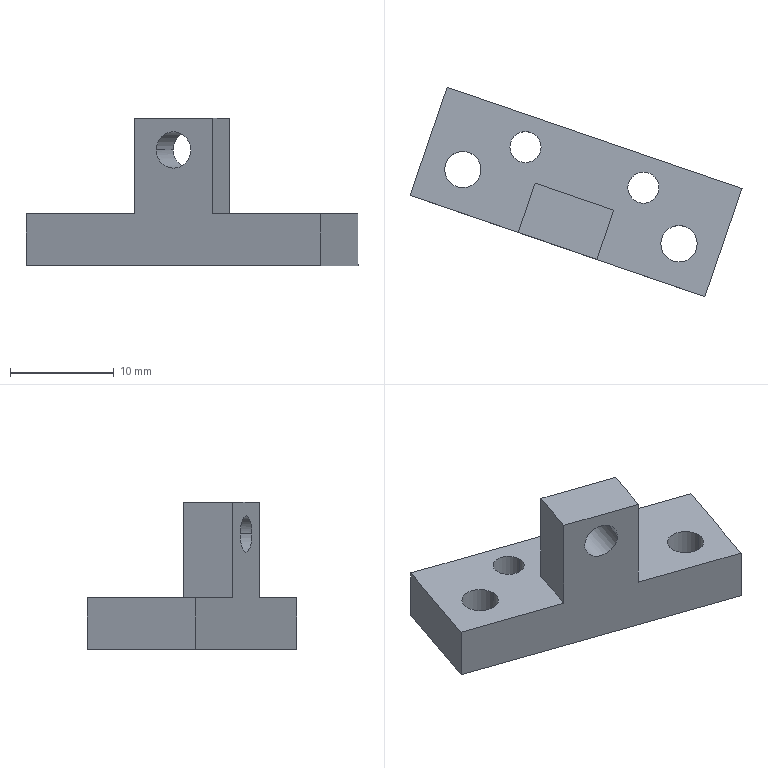Part | SolidWorks | features Cut 7, ICE 5, Extrusion 1, HoleWzd 1 | 1 solid | 20 faces | box 31.948 x 20.133 x 14.168 mm | volume 1802 mm3 | cylinder 10 | plane 10 | commonest cylinder face diameters 3.5 x6 3 x4
STEP:
#1=CARTESIAN_POINT('',(-193.386,195.318,0.));
#2=VERTEX_POINT('',#1);
#3=CARTESIAN_POINT('',(-189.886,195.318,0.));
#4=VERTEX_POINT('',#3);
#5=CARTESIAN_POINT('',(-191.636,195.318,0.));
#6=DIRECTION('',(0.,0.,1.));
#7=DIRECTION('',(1.,0.,0.));
#8=AXIS2_PLACEMENT_3D('',#5,#6,#7);
#9=CIRCLE('',#8,1.75);
#10=EDGE_CURVE('',#2,#4,#9,.T.);
#11=ORIENTED_EDGE('',*,*,#10,.F.);
#12=CARTESIAN_POINT('',(-193.386,195.318,5.));
#13=VERTEX_POINT('',#12);
#14=CARTESIAN_POINT('',(-193.386,195.318,5.));
#15=DIRECTION('',(0.,0.,1.));
#16=VECTOR('',#15,1000.);
#17=LINE('',#14,#16);
#18=EDGE_CURVE('',#2,#13,#17,.T.);
#19=ORIENTED_EDGE('',*,*,#18,.T.);
#20=CARTESIAN_POINT('',(-189.886,195.318,5.));
#21=VERTEX_POINT('',#20);
#22=CARTESIAN_POINT('',(-191.636,195.318,5.));
#23=DIRECTION('',(0.,0.,1.));
#24=DIRECTION('',(1.,0.,0.));
#25=AXIS2_PLACEMENT_3D('',#22,#23,#24);
#26=CIRCLE('',#25,1.75);
#27=EDGE_CURVE('',#13,#21,#26,.T.);
#28=ORIENTED_EDGE('',*,*,#27,.T.);
#29=CARTESIAN_POINT('',(-189.886,195.318,5.));
#30=DIRECTION('',(0.,0.,1.));
#31=VECTOR('',#30,1000.);
#32=LINE('',#29,#31);
#33=EDGE_CURVE('',#4,#21,#32,.T.);
#34=ORIENTED_EDGE('',*,*,#33,.F.);
#35=EDGE_LOOP('',(#11,#19,#28,#34));
#36=FACE_OUTER_BOUND('',#35,.T.);
#37=CARTESIAN_POINT('',(-191.636,195.318,5.));
#38=DIRECTION('',(0.,0.,1.));
#39=DIRECTION('',(1.,0.,0.));
#40=AXIS2_PLACEMENT_3D('',#37,#38,#39);
#41=CYLINDRICAL_SURFACE('',#40,1.75);
#42=ADVANCED_FACE('',(#36),#41,.F.);
#43=CARTESIAN_POINT('',(-172.577,188.179,0.));
#44=VERTEX_POINT('',#43);
#45=CARTESIAN_POINT('',(-169.077,188.179,0.));
#46=VERTEX_POINT('',#45);
#47=CARTESIAN_POINT('',(-170.827,188.179,0.));
#48=DIRECTION('',(0.,0.,1.));
#49=DIRECTION('',(1.,0.,0.));
#50=AXIS2_PLACEMENT_3D('',#47,#48,#49);
#51=CIRCLE('',#50,1.75);
#52=EDGE_CURVE('',#44,#46,#51,.T.);
#53=ORIENTED_EDGE('',*,*,#52,.F.);
#54=CARTESIAN_POINT('',(-172.577,188.179,5.));
#55=VERTEX_POINT('',#54);
#56=CARTESIAN_POINT('',(-172.577,188.179,5.));
#57=DIRECTION('',(0.,0.,1.));
#58=VECTOR('',#57,1000.);
#59=LINE('',#56,#58);
#60=EDGE_CURVE('',#44,#55,#59,.T.);
#61=ORIENTED_EDGE('',*,*,#60,.T.);
#62=CARTESIAN_POINT('',(-169.077,188.179,5.));
#63=VERTEX_POINT('',#62);
#64=CARTESIAN_POINT('',(-170.827,188.179,5.));
#65=DIRECTION('',(0.,0.,1.));
#66=DIRECTION('',(1.,0.,0.));
#67=AXIS2_PLACEMENT_3D('',#64,#65,#66);
#68=CIRCLE('',#67,1.75);
#69=EDGE_CURVE('',#55,#63,#68,.T.);
#70=ORIENTED_EDGE('',*,*,#69,.T.);
#71=CARTESIAN_POINT('',(-169.077,188.179,5.));
#72=DIRECTION('',(0.,0.,1.));
#73=VECTOR('',#72,1000.);
#74=LINE('',#71,#73);
#75=EDGE_CURVE('',#46,#63,#74,.T.);
#76=ORIENTED_EDGE('',*,*,#75,.F.);
#77=EDGE_LOOP('',(#53,#61,#70,#76));
#78=FACE_OUTER_BOUND('',#77,.T.);
#79=CARTESIAN_POINT('',(-170.827,188.179,5.));
#80=DIRECTION('',(0.,0.,1.));
#81=DIRECTION('',(1.,0.,0.));
#82=AXIS2_PLACEMENT_3D('',#79,#80,#81);
#83=CYLINDRICAL_SURFACE('',#82,1.75);
#84=ADVANCED_FACE('',(#78),#83,.F.);
#85=CARTESIAN_POINT('',(-175.758,193.585,0.));
#86=VERTEX_POINT('',#85);
#87=CARTESIAN_POINT('',(-172.758,193.585,0.));
#88=VERTEX_POINT('',#87);
#89=CARTESIAN_POINT('',(-174.258,193.585,0.));
#90=DIRECTION('',(0.,0.,1.));
#91=DIRECTION('',(1.,0.,0.));
#92=AXIS2_PLACEMENT_3D('',#89,#90,#91);
#93=CIRCLE('',#92,1.5);
#94=EDGE_CURVE('',#86,#88,#93,.T.);
#95=ORIENTED_EDGE('',*,*,#94,.F.);
#96=CARTESIAN_POINT('',(-175.758,193.585,5.));
#97=VERTEX_POINT('',#96);
#98=CARTESIAN_POINT('',(-175.758,193.585,0.));
#99=DIRECTION('',(0.,0.,1.));
#100=VECTOR('',#99,1000.);
#101=LINE('',#98,#100);
#102=EDGE_CURVE('',#86,#97,#101,.T.);
#103=ORIENTED_EDGE('',*,*,#102,.T.);
#104=CARTESIAN_POINT('',(-172.758,193.585,5.));
#105=VERTEX_POINT('',#104);
#106=CARTESIAN_POINT('',(-174.258,193.585,5.));
#107=DIRECTION('',(0.,0.,1.));
#108=DIRECTION('',(1.,0.,0.));
#109=AXIS2_PLACEMENT_3D('',#106,#107,#108);
#110=CIRCLE('',#109,1.5);
#111=EDGE_CURVE('',#97,#105,#110,.T.);
#112=ORIENTED_EDGE('',*,*,#111,.T.);
#113=CARTESIAN_POINT('',(-172.758,193.585,0.));
#114=DIRECTION('',(0.,0.,1.));
#115=VECTOR('',#114,1000.);
#116=LINE('',#113,#115);
#117=EDGE_CURVE('',#88,#105,#116,.T.);
#118=ORIENTED_EDGE('',*,*,#117,.F.);
#119=EDGE_LOOP('',(#95,#103,#112,#118));
#120=FACE_OUTER_BOUND('',#119,.T.);
#121=CARTESIAN_POINT('',(-174.258,193.585,0.));
#122=DIRECTION('',(0.,0.,1.));
#123=DIRECTION('',(1.,0.,0.));
#124=AXIS2_PLACEMENT_3D('',#121,#122,#123);
#125=CYLINDRICAL_SURFACE('',#124,1.5);
#126=ADVANCED_FACE('',(#120),#125,.F.);
#127=CARTESIAN_POINT('',(-187.109,197.479,0.));
#128=VERTEX_POINT('',#127);
#129=CARTESIAN_POINT('',(-184.109,197.479,0.));
#130=VERTEX_POINT('',#129);
#131=CARTESIAN_POINT('',(-185.609,197.479,0.));
#132=DIRECTION('',(0.,0.,1.));
#133=DIRECTION('',(1.,0.,0.));
#134=AXIS2_PLACEMENT_3D('',#131,#132,#133);
#135=CIRCLE('',#134,1.5);
#136=EDGE_CURVE('',#128,#130,#135,.T.);
#137=ORIENTED_EDGE('',*,*,#136,.F.);
#138=CARTESIAN_POINT('',(-187.109,197.479,5.));
#139=VERTEX_POINT('',#138);
#140=CARTESIAN_POINT('',(-187.109,197.479,0.));
#141=DIRECTION('',(0.,0.,1.));
#142=VECTOR('',#141,1000.);
#143=LINE('',#140,#142);
#144=EDGE_CURVE('',#128,#139,#143,.T.);
#145=ORIENTED_EDGE('',*,*,#144,.T.);
#146=CARTESIAN_POINT('',(-184.109,197.479,5.));
#147=VERTEX_POINT('',#146);
#148=CARTESIAN_POINT('',(-185.609,197.479,5.));
#149=DIRECTION('',(0.,0.,1.));
#150=DIRECTION('',(1.,0.,0.));
#151=AXIS2_PLACEMENT_3D('',#148,#149,#150);
#152=CIRCLE('',#151,1.5);
#153=EDGE_CURVE('',#139,#147,#152,.T.);
#154=ORIENTED_EDGE('',*,*,#153,.T.);
#155=CARTESIAN_POINT('',(-184.109,197.479,0.));
#156=DIRECTION('',(0.,0.,1.));
#157=VECTOR('',#156,1000.);
#158=LINE('',#155,#157);
#159=EDGE_CURVE('',#130,#147,#158,.T.);
#160=ORIENTED_EDGE('',*,*,#159,.F.);
#161=EDGE_LOOP('',(#137,#145,#154,#160));
#162=FACE_OUTER_BOUND('',#161,.T.);
#163=CARTESIAN_POINT('',(-185.609,197.479,0.));
#164=DIRECTION('',(0.,0.,1.));
#165=DIRECTION('',(1.,0.,0.));
#166=AXIS2_PLACEMENT_3D('',#163,#164,#165);
#167=CYLINDRICAL_SURFACE('',#166,1.5);
#168=ADVANCED_FACE('',(#162),#167,.F.);
#169=CARTESIAN_POINT('',(-180.87,187.396,11.129));
#170=VERTEX_POINT('',#169);
#171=CARTESIAN_POINT('',(-184.181,188.532,11.129));
#172=VERTEX_POINT('',#171);
#173=CARTESIAN_POINT('',(-180.87,187.396,11.129));
#174=CARTESIAN_POINT('',(-180.87,187.396,7.629));
#175=CARTESIAN_POINT('',(-184.181,188.532,7.629));
#176=CARTESIAN_POINT('',(-184.181,188.532,11.129));
#177=(BOUNDED_CURVE()B_SPLINE_CURVE(3,(#173,#174,#175,#176),.UNSPECIFIED.,.F.,.F.)B_SPLINE_CURVE_WITH_KNOTS((4,4),(3.142,6.283),.UNSPECIFIED.)CURVE()GEOMETRIC_REPRESENTATION_ITEM()RATIONAL_B_SPLINE_CURVE((1.,0.3333,0.3333,1.))REPRESENTATION_ITEM(''));
#178=EDGE_CURVE('',#170,#172,#177,.T.);
#179=ORIENTED_EDGE('',*,*,#178,.F.);
#180=CARTESIAN_POINT('',(-179.249,192.129,11.129));
#181=VERTEX_POINT('',#180);
#182=CARTESIAN_POINT('',(-183.852,178.691,11.129));
#183=DIRECTION('',(0.324,0.946,0.));
#184=VECTOR('',#183,1000.);
#185=LINE('',#182,#184);
#186=EDGE_CURVE('',#170,#181,#185,.T.);
#187=ORIENTED_EDGE('',*,*,#186,.T.);
#188=CARTESIAN_POINT('',(-182.56,193.263,11.129));
#189=VERTEX_POINT('',#188);
#190=CARTESIAN_POINT('',(-180.905,192.696,11.129));
#191=DIRECTION('',(0.324,0.946,0.));
#192=DIRECTION('',(-0.946,0.324,0.));
#193=AXIS2_PLACEMENT_3D('',#190,#191,#192);
#194=CIRCLE('',#193,1.75);
#195=EDGE_CURVE('',#181,#189,#194,.T.);
#196=ORIENTED_EDGE('',*,*,#195,.T.);
#197=CARTESIAN_POINT('',(-187.163,179.825,11.129));
#198=DIRECTION('',(0.324,0.946,0.));
#199=VECTOR('',#198,1000.);
#200=LINE('',#197,#199);
#201=EDGE_CURVE('',#172,#189,#200,.T.);
#202=ORIENTED_EDGE('',*,*,#201,.F.);
#203=EDGE_LOOP('',(#179,#187,#196,#202));
#204=FACE_OUTER_BOUND('',#203,.T.);
#205=CARTESIAN_POINT('',(-185.507,179.258,11.129));
#206=DIRECTION('',(0.324,0.946,0.));
#207=DIRECTION('',(-0.946,0.324,0.));
#208=AXIS2_PLACEMENT_3D('',#205,#206,#207);
#209=CYLINDRICAL_SURFACE('',#208,1.75);
#210=ADVANCED_FACE('',(#204),#209,.F.);
#211=CARTESIAN_POINT('',(-191.636,195.318,5.));
#212=DIRECTION('',(0.,0.,1.));
#213=DIRECTION('',(1.,0.,0.));
#214=AXIS2_PLACEMENT_3D('',#211,#212,#213);
#215=CIRCLE('',#214,1.75);
#216=EDGE_CURVE('',#21,#13,#215,.T.);
#217=ORIENTED_EDGE('',*,*,#216,.F.);
#218=ORIENTED_EDGE('',*,*,#27,.F.);
#219=EDGE_LOOP('',(#217,#218));
#220=FACE_BOUND('',#219,.T.);
#221=CARTESIAN_POINT('',(-170.827,188.179,5.));
#222=DIRECTION('',(0.,0.,1.));
#223=DIRECTION('',(1.,0.,0.));
#224=AXIS2_PLACEMENT_3D('',#221,#222,#223);
#225=CIRCLE('',#224,1.75);
#226=EDGE_CURVE('',#63,#55,#225,.T.);
#227=ORIENTED_EDGE('',*,*,#226,.F.);
#228=ORIENTED_EDGE('',*,*,#69,.F.);
#229=EDGE_LOOP('',(#227,#228));
#230=FACE_BOUND('',#229,.T.);
#231=CARTESIAN_POINT('',(-174.258,193.585,5.));
#232=DIRECTION('',(0.,0.,1.));
#233=DIRECTION('',(1.,0.,0.));
#234=AXIS2_PLACEMENT_3D('',#231,#232,#233);
#235=CIRCLE('',#234,1.5);
#236=EDGE_CURVE('',#105,#97,#235,.T.);
#237=ORIENTED_EDGE('',*,*,#236,.F.);
#238=ORIENTED_EDGE('',*,*,#111,.F.);
#239=EDGE_LOOP('',(#237,#238));
#240=FACE_BOUND('',#239,.T.);
#241=CARTESIAN_POINT('',(-185.609,197.479,5.));
#242=DIRECTION('',(0.,0.,1.));
#243=DIRECTION('',(1.,0.,0.));
#244=AXIS2_PLACEMENT_3D('',#241,#242,#243);
#245=CIRCLE('',#244,1.5);
#246=EDGE_CURVE('',#147,#139,#245,.T.);
#247=ORIENTED_EDGE('',*,*,#246,.F.);
#248=ORIENTED_EDGE('',*,*,#153,.F.);
#249=EDGE_LOOP('',(#247,#248));
#250=FACE_BOUND('',#249,.T.);
#251=CARTESIAN_POINT('',(-178.742,186.666,5.));
#252=VERTEX_POINT('',#251);
#253=CARTESIAN_POINT('',(-177.12,191.399,5.));
#254=VERTEX_POINT('',#253);
#255=CARTESIAN_POINT('',(-181.723,177.962,5.));
#256=DIRECTION('',(0.324,0.946,0.));
#257=VECTOR('',#256,1000.);
#258=LINE('',#255,#257);
#259=EDGE_CURVE('',#252,#254,#258,.T.);
#260=ORIENTED_EDGE('',*,*,#259,.F.);
#261=CARTESIAN_POINT('',(-168.341,183.098,5.));
#262=VERTEX_POINT('',#261);
#263=CARTESIAN_POINT('',(-196.718,192.833,5.));
#264=DIRECTION('',(0.9459,-0.3245,0.));
#265=VECTOR('',#264,1000.);
#266=LINE('',#263,#265);
#267=EDGE_CURVE('',#252,#262,#266,.T.);
#268=ORIENTED_EDGE('',*,*,#267,.T.);
#269=CARTESIAN_POINT('',(-164.769,193.51,5.));
#270=VERTEX_POINT('',#269);
#271=CARTESIAN_POINT('',(-164.772,193.503,5.));
#272=DIRECTION('',(0.3245,0.9459,0.));
#273=VECTOR('',#272,1000.);
#274=LINE('',#271,#273);
#275=EDGE_CURVE('',#262,#270,#274,.T.);
#276=ORIENTED_EDGE('',*,*,#275,.T.);
#277=CARTESIAN_POINT('',(-193.151,203.231,5.));
#278=VERTEX_POINT('',#277);
#279=CARTESIAN_POINT('',(-153.192,189.544,5.));
#280=DIRECTION('',(-0.946,0.324,0.));
#281=VECTOR('',#280,1000.);
#282=LINE('',#279,#281);
#283=EDGE_CURVE('',#270,#278,#282,.T.);
#284=ORIENTED_EDGE('',*,*,#283,.T.);
#285=CARTESIAN_POINT('',(-196.718,192.833,5.));
#286=VERTEX_POINT('',#285);
#287=CARTESIAN_POINT('',(-193.148,203.238,5.));
#288=DIRECTION('',(-0.3245,-0.9459,0.));
#289=VECTOR('',#288,1000.);
#290=LINE('',#287,#289);
#291=EDGE_CURVE('',#278,#286,#290,.T.);
#292=ORIENTED_EDGE('',*,*,#291,.T.);
#293=CARTESIAN_POINT('',(-186.309,189.262,5.));
#294=VERTEX_POINT('',#293);
#295=CARTESIAN_POINT('',(-196.718,192.833,5.));
#296=DIRECTION('',(0.9459,-0.3245,0.));
#297=VECTOR('',#296,1000.);
#298=LINE('',#295,#297);
#299=EDGE_CURVE('',#286,#294,#298,.T.);
#300=ORIENTED_EDGE('',*,*,#299,.T.);
#301=CARTESIAN_POINT('',(-184.689,193.992,5.));
#302=VERTEX_POINT('',#301);
#303=CARTESIAN_POINT('',(-189.291,180.554,5.));
#304=DIRECTION('',(0.324,0.946,0.));
#305=VECTOR('',#304,1000.);
#306=LINE('',#303,#305);
#307=EDGE_CURVE('',#294,#302,#306,.T.);
#308=ORIENTED_EDGE('',*,*,#307,.T.);
#309=CARTESIAN_POINT('',(-155.136,183.869,5.));
#310=DIRECTION('',(-0.946,0.324,0.));
#311=VECTOR('',#310,1000.);
#312=LINE('',#309,#311);
#313=EDGE_CURVE('',#254,#302,#312,.T.);
#314=ORIENTED_EDGE('',*,*,#313,.F.);
#315=EDGE_LOOP('',(#260,#268,#276,#284,#292,#300,#308,#314));
#316=FACE_OUTER_BOUND('',#315,.T.);
#317=CARTESIAN_POINT('',(0.,0.,5.));
#318=DIRECTION('',(0.,0.,1.));
#319=DIRECTION('',(1.,0.,0.));
#320=AXIS2_PLACEMENT_3D('',#317,#318,#319);
#321=PLANE('',#320);
#322=ADVANCED_FACE('',(#220,#230,#240,#250,#316),#321,.T.);
#323=CARTESIAN_POINT('',(-193.151,203.231,0.));
#324=VERTEX_POINT('',#323);
#325=CARTESIAN_POINT('',(-196.718,192.833,0.));
#326=VERTEX_POINT('',#325);
#327=CARTESIAN_POINT('',(-193.148,203.238,0.));
#328=DIRECTION('',(-0.3245,-0.9459,0.));
#329=VECTOR('',#328,1000.);
#330=LINE('',#327,#329);
#331=EDGE_CURVE('',#324,#326,#330,.T.);
#332=ORIENTED_EDGE('',*,*,#331,.T.);
#333=CARTESIAN_POINT('',(-196.718,192.833,0.));
#334=DIRECTION('',(0.,0.,1.));
#335=VECTOR('',#334,1000.);
#336=LINE('',#333,#335);
#337=EDGE_CURVE('',#326,#286,#336,.T.);
#338=ORIENTED_EDGE('',*,*,#337,.T.);
#339=ORIENTED_EDGE('',*,*,#291,.F.);
#340=CARTESIAN_POINT('',(-193.151,203.231,0.));
#341=DIRECTION('',(0.,0.,-1.));
#342=VECTOR('',#341,1000.);
#343=LINE('',#340,#342);
#344=EDGE_CURVE('',#278,#324,#343,.T.);
#345=ORIENTED_EDGE('',*,*,#344,.T.);
#346=EDGE_LOOP('',(#332,#338,#339,#345));
#347=FACE_OUTER_BOUND('',#346,.T.);
#348=CARTESIAN_POINT('',(-193.148,203.238,5.));
#349=DIRECTION('',(0.9459,-0.3245,0.));
#350=DIRECTION('',(0.3245,0.9459,0.));
#351=AXIS2_PLACEMENT_3D('',#348,#349,#350);
#352=PLANE('',#351);
#353=ADVANCED_FACE('',(#347),#352,.F.);
#354=CARTESIAN_POINT('',(-164.769,193.51,0.));
#355=VERTEX_POINT('',#354);
#356=CARTESIAN_POINT('',(-164.769,193.51,5.));
#357=DIRECTION('',(0.,0.,1.));
#358=VECTOR('',#357,1000.);
#359=LINE('',#356,#358);
#360=EDGE_CURVE('',#355,#270,#359,.T.);
#361=ORIENTED_EDGE('',*,*,#360,.T.);
#362=ORIENTED_EDGE('',*,*,#275,.F.);
#363=CARTESIAN_POINT('',(-168.341,183.098,0.));
#364=VERTEX_POINT('',#363);
#365=CARTESIAN_POINT('',(-168.341,183.098,5.));
#366=DIRECTION('',(0.,0.,-1.));
#367=VECTOR('',#366,1000.);
#368=LINE('',#365,#367);
#369=EDGE_CURVE('',#262,#364,#368,.T.);
#370=ORIENTED_EDGE('',*,*,#369,.T.);
#371=CARTESIAN_POINT('',(-164.772,193.503,0.));
#372=DIRECTION('',(0.3245,0.9459,0.));
#373=VECTOR('',#372,1000.);
#374=LINE('',#371,#373);
#375=EDGE_CURVE('',#364,#355,#374,.T.);
#376=ORIENTED_EDGE('',*,*,#375,.T.);
#377=EDGE_LOOP('',(#361,#362,#370,#376));
#378=FACE_OUTER_BOUND('',#377,.T.);
#379=CARTESIAN_POINT('',(-164.772,193.503,5.));
#380=DIRECTION('',(-0.9459,0.3245,0.));
#381=DIRECTION('',(-0.3245,-0.9459,0.));
#382=AXIS2_PLACEMENT_3D('',#379,#380,#381);
#383=PLANE('',#382);
#384=ADVANCED_FACE('',(#378),#383,.F.);
#385=CARTESIAN_POINT('',(-191.636,195.318,0.));
#386=DIRECTION('',(0.,0.,1.));
#387=DIRECTION('',(1.,0.,0.));
#388=AXIS2_PLACEMENT_3D('',#385,#386,#387);
#389=CIRCLE('',#388,1.75);
#390=EDGE_CURVE('',#4,#2,#389,.T.);
#391=ORIENTED_EDGE('',*,*,#390,.T.);
#392=ORIENTED_EDGE('',*,*,#10,.T.);
#393=EDGE_LOOP('',(#391,#392));
#394=FACE_BOUND('',#393,.T.);
#395=CARTESIAN_POINT('',(-170.827,188.179,0.));
#396=DIRECTION('',(0.,0.,1.));
#397=DIRECTION('',(1.,0.,0.));
#398=AXIS2_PLACEMENT_3D('',#395,#396,#397);
#399=CIRCLE('',#398,1.75);
#400=EDGE_CURVE('',#46,#44,#399,.T.);
#401=ORIENTED_EDGE('',*,*,#400,.T.);
#402=ORIENTED_EDGE('',*,*,#52,.T.);
#403=EDGE_LOOP('',(#401,#402));
#404=FACE_BOUND('',#403,.T.);
#405=CARTESIAN_POINT('',(-174.258,193.585,0.));
#406=DIRECTION('',(0.,0.,1.));
#407=DIRECTION('',(1.,0.,0.));
#408=AXIS2_PLACEMENT_3D('',#405,#406,#407);
#409=CIRCLE('',#408,1.5);
#410=EDGE_CURVE('',#88,#86,#409,.T.);
#411=ORIENTED_EDGE('',*,*,#410,.T.);
#412=ORIENTED_EDGE('',*,*,#94,.T.);
#413=EDGE_LOOP('',(#411,#412));
#414=FACE_BOUND('',#413,.T.);
#415=CARTESIAN_POINT('',(-185.609,197.479,0.));
#416=DIRECTION('',(0.,0.,1.));
#417=DIRECTION('',(1.,0.,0.));
#418=AXIS2_PLACEMENT_3D('',#415,#416,#417);
#419=CIRCLE('',#418,1.5);
#420=EDGE_CURVE('',#130,#128,#419,.T.);
#421=ORIENTED_EDGE('',*,*,#420,.T.);
#422=ORIENTED_EDGE('',*,*,#136,.T.);
#423=EDGE_LOOP('',(#421,#422));
#424=FACE_BOUND('',#423,.T.);
#425=ORIENTED_EDGE('',*,*,#331,.F.);
#426=CARTESIAN_POINT('',(-160.125,191.919,0.));
#427=DIRECTION('',(-0.946,0.324,0.));
#428=VECTOR('',#427,1000.);
#429=LINE('',#426,#428);
#430=EDGE_CURVE('',#355,#324,#429,.T.);
#431=ORIENTED_EDGE('',*,*,#430,.F.);
#432=ORIENTED_EDGE('',*,*,#375,.F.);
#433=CARTESIAN_POINT('',(-168.341,183.098,0.));
#434=DIRECTION('',(-0.9459,0.3245,0.));
#435=VECTOR('',#434,1000.);
#436=LINE('',#433,#435);
#437=EDGE_CURVE('',#364,#326,#436,.T.);
#438=ORIENTED_EDGE('',*,*,#437,.T.);
#439=EDGE_LOOP('',(#425,#431,#432,#438));
#440=FACE_OUTER_BOUND('',#439,.T.);
#441=CARTESIAN_POINT('',(0.,0.,0.));
#442=DIRECTION('',(0.,0.,1.));
#443=DIRECTION('',(1.,0.,0.));
#444=AXIS2_PLACEMENT_3D('',#441,#442,#443);
#445=PLANE('',#444);
#446=ADVANCED_FACE('',(#394,#404,#414,#424,#440),#445,.F.);
#447=CARTESIAN_POINT('',(-184.181,188.532,11.129));
#448=CARTESIAN_POINT('',(-184.181,188.532,14.629));
#449=CARTESIAN_POINT('',(-180.87,187.396,14.629));
#450=CARTESIAN_POINT('',(-180.87,187.396,11.129));
#451=(BOUNDED_CURVE()B_SPLINE_CURVE(3,(#447,#448,#449,#450),.UNSPECIFIED.,.F.,.F.)B_SPLINE_CURVE_WITH_KNOTS((4,4),(0.,3.142),.UNSPECIFIED.)CURVE()GEOMETRIC_REPRESENTATION_ITEM()RATIONAL_B_SPLINE_CURVE((1.,0.3333,0.3333,1.))REPRESENTATION_ITEM(''));
#452=EDGE_CURVE('',#172,#170,#451,.T.);
#453=ORIENTED_EDGE('',*,*,#452,.T.);
#454=ORIENTED_EDGE('',*,*,#178,.T.);
#455=EDGE_LOOP('',(#453,#454));
#456=FACE_BOUND('',#455,.T.);
#457=ORIENTED_EDGE('',*,*,#299,.F.);
#458=ORIENTED_EDGE('',*,*,#337,.F.);
#459=ORIENTED_EDGE('',*,*,#437,.F.);
#460=ORIENTED_EDGE('',*,*,#369,.F.);
#461=ORIENTED_EDGE('',*,*,#267,.F.);
#462=CARTESIAN_POINT('',(-178.742,186.666,14.168));
#463=VERTEX_POINT('',#462);
#464=CARTESIAN_POINT('',(-178.742,186.666,5.));
#465=DIRECTION('',(0.,0.,-1.));
#466=VECTOR('',#465,1000.);
#467=LINE('',#464,#466);
#468=EDGE_CURVE('',#463,#252,#467,.T.);
#469=ORIENTED_EDGE('',*,*,#468,.F.);
#470=CARTESIAN_POINT('',(-186.309,189.262,14.168));
#471=VERTEX_POINT('',#470);
#472=CARTESIAN_POINT('',(-178.736,186.664,14.168));
#473=DIRECTION('',(0.9459,-0.3245,0.));
#474=VECTOR('',#473,1000.);
#475=LINE('',#472,#474);
#476=EDGE_CURVE('',#471,#463,#475,.T.);
#477=ORIENTED_EDGE('',*,*,#476,.F.);
#478=CARTESIAN_POINT('',(-186.309,189.262,14.168));
#479=DIRECTION('',(0.,0.,1.));
#480=VECTOR('',#479,1000.);
#481=LINE('',#478,#480);
#482=EDGE_CURVE('',#294,#471,#481,.T.);
#483=ORIENTED_EDGE('',*,*,#482,.F.);
#484=EDGE_LOOP('',(#457,#458,#459,#460,#461,#469,#477,#483));
#485=FACE_OUTER_BOUND('',#484,.T.);
#486=CARTESIAN_POINT('',(38.474,112.147,0.));
#487=DIRECTION('',(0.3245,0.9459,0.));
#488=DIRECTION('',(-0.9459,0.3245,0.));
#489=AXIS2_PLACEMENT_3D('',#486,#487,#488);
#490=PLANE('',#489);
#491=ADVANCED_FACE('',(#456,#485),#490,.F.);
#492=CARTESIAN_POINT('',(-180.905,192.696,11.129));
#493=DIRECTION('',(0.324,0.946,0.));
#494=DIRECTION('',(-0.946,0.324,0.));
#495=AXIS2_PLACEMENT_3D('',#492,#493,#494);
#496=CIRCLE('',#495,1.75);
#497=EDGE_CURVE('',#189,#181,#496,.T.);
#498=ORIENTED_EDGE('',*,*,#497,.F.);
#499=ORIENTED_EDGE('',*,*,#195,.F.);
#500=EDGE_LOOP('',(#498,#499));
#501=FACE_BOUND('',#500,.T.);
#502=CARTESIAN_POINT('',(-184.689,193.992,14.168));
#503=VERTEX_POINT('',#502);
#504=CARTESIAN_POINT('',(-184.689,193.992,14.168));
#505=DIRECTION('',(0.,0.,-1.));
#506=VECTOR('',#505,1000.);
#507=LINE('',#504,#506);
#508=EDGE_CURVE('',#503,#302,#507,.T.);
#509=ORIENTED_EDGE('',*,*,#508,.F.);
#510=CARTESIAN_POINT('',(-177.12,191.399,14.168));
#511=VERTEX_POINT('',#510);
#512=CARTESIAN_POINT('',(-155.136,183.869,14.168));
#513=DIRECTION('',(-0.946,0.324,0.));
#514=VECTOR('',#513,1000.);
#515=LINE('',#512,#514);
#516=EDGE_CURVE('',#511,#503,#515,.T.);
#517=ORIENTED_EDGE('',*,*,#516,.F.);
#518=CARTESIAN_POINT('',(-177.12,191.399,14.168));
#519=DIRECTION('',(0.,0.,1.));
#520=VECTOR('',#519,1000.);
#521=LINE('',#518,#520);
#522=EDGE_CURVE('',#254,#511,#521,.T.);
#523=ORIENTED_EDGE('',*,*,#522,.F.);
#524=ORIENTED_EDGE('',*,*,#313,.T.);
#525=EDGE_LOOP('',(#509,#517,#523,#524));
#526=FACE_OUTER_BOUND('',#525,.T.);
#527=CARTESIAN_POINT('',(-155.136,183.869,5.));
#528=DIRECTION('',(0.324,0.946,0.));
#529=DIRECTION('',(-0.946,0.324,0.));
#530=AXIS2_PLACEMENT_3D('',#527,#528,#529);
#531=PLANE('',#530);
#532=ADVANCED_FACE('',(#501,#526),#531,.T.);
#533=ORIENTED_EDGE('',*,*,#516,.T.);
#534=CARTESIAN_POINT('',(-224.765,76.986,14.168));
#535=DIRECTION('',(-0.324,-0.946,0.));
#536=VECTOR('',#535,1000.);
#537=LINE('',#534,#536);
#538=EDGE_CURVE('',#503,#471,#537,.T.);
#539=ORIENTED_EDGE('',*,*,#538,.T.);
#540=ORIENTED_EDGE('',*,*,#476,.T.);
#541=CARTESIAN_POINT('',(-217.197,74.394,14.168));
#542=DIRECTION('',(0.324,0.946,0.));
#543=VECTOR('',#542,1000.);
#544=LINE('',#541,#543);
#545=EDGE_CURVE('',#463,#511,#544,.T.);
#546=ORIENTED_EDGE('',*,*,#545,.T.);
#547=EDGE_LOOP('',(#533,#539,#540,#546));
#548=FACE_OUTER_BOUND('',#547,.T.);
#549=CARTESIAN_POINT('',(0.,0.,14.168));
#550=DIRECTION('',(0.,0.,-1.));
#551=DIRECTION('',(-1.,0.,0.));
#552=AXIS2_PLACEMENT_3D('',#549,#550,#551);
#553=PLANE('',#552);
#554=ADVANCED_FACE('',(#548),#553,.F.);
#555=ORIENTED_EDGE('',*,*,#283,.F.);
#556=ORIENTED_EDGE('',*,*,#360,.F.);
#557=ORIENTED_EDGE('',*,*,#430,.T.);
#558=ORIENTED_EDGE('',*,*,#344,.F.);
#559=EDGE_LOOP('',(#555,#556,#557,#558));
#560=FACE_OUTER_BOUND('',#559,.T.);
#561=CARTESIAN_POINT('',(-160.125,191.919,5.));
#562=DIRECTION('',(-0.324,-0.946,0.));
#563=DIRECTION('',(0.946,-0.324,0.));
#564=AXIS2_PLACEMENT_3D('',#561,#562,#563);
#565=PLANE('',#564);
#566=ADVANCED_FACE('',(#560),#565,.F.);
#567=ORIENTED_EDGE('',*,*,#545,.F.);
#568=ORIENTED_EDGE('',*,*,#468,.T.);
#569=ORIENTED_EDGE('',*,*,#259,.T.);
#570=ORIENTED_EDGE('',*,*,#522,.T.);
#571=EDGE_LOOP('',(#567,#568,#569,#570));
#572=FACE_OUTER_BOUND('',#571,.T.);
#573=CARTESIAN_POINT('',(-181.723,177.962,14.168));
#574=DIRECTION('',(-0.946,0.324,0.));
#575=DIRECTION('',(-0.324,-0.946,0.));
#576=AXIS2_PLACEMENT_3D('',#573,#574,#575);
#577=PLANE('',#576);
#578=ADVANCED_FACE('',(#572),#577,.F.);
#579=ORIENTED_EDGE('',*,*,#307,.F.);
#580=ORIENTED_EDGE('',*,*,#482,.T.);
#581=ORIENTED_EDGE('',*,*,#538,.F.);
#582=ORIENTED_EDGE('',*,*,#508,.T.);
#583=EDGE_LOOP('',(#579,#580,#581,#582));
#584=FACE_OUTER_BOUND('',#583,.T.);
#585=CARTESIAN_POINT('',(-189.291,180.554,14.168));
#586=DIRECTION('',(0.946,-0.324,0.));
#587=DIRECTION('',(0.324,0.946,0.));
#588=AXIS2_PLACEMENT_3D('',#585,#586,#587);
#589=PLANE('',#588);
#590=ADVANCED_FACE('',(#584),#589,.F.);
#591=ORIENTED_EDGE('',*,*,#186,.F.);
#592=ORIENTED_EDGE('',*,*,#452,.F.);
#593=ORIENTED_EDGE('',*,*,#201,.T.);
#594=ORIENTED_EDGE('',*,*,#497,.T.);
#595=EDGE_LOOP('',(#591,#592,#593,#594));
#596=FACE_OUTER_BOUND('',#595,.T.);
#597=CARTESIAN_POINT('',(-185.507,179.258,11.129));
#598=DIRECTION('',(0.324,0.946,0.));
#599=DIRECTION('',(-0.946,0.324,0.));
#600=AXIS2_PLACEMENT_3D('',#597,#598,#599);
#601=CYLINDRICAL_SURFACE('',#600,1.75);
#602=ADVANCED_FACE('',(#596),#601,.F.);
#603=ORIENTED_EDGE('',*,*,#144,.F.);
#604=ORIENTED_EDGE('',*,*,#420,.F.);
#605=ORIENTED_EDGE('',*,*,#159,.T.);
#606=ORIENTED_EDGE('',*,*,#246,.T.);
#607=EDGE_LOOP('',(#603,#604,#605,#606));
#608=FACE_OUTER_BOUND('',#607,.T.);
#609=CARTESIAN_POINT('',(-185.609,197.479,0.));
#610=DIRECTION('',(0.,0.,1.));
#611=DIRECTION('',(1.,0.,0.));
#612=AXIS2_PLACEMENT_3D('',#609,#610,#611);
#613=CYLINDRICAL_SURFACE('',#612,1.5);
#614=ADVANCED_FACE('',(#608),#613,.F.);
#615=ORIENTED_EDGE('',*,*,#102,.F.);
#616=ORIENTED_EDGE('',*,*,#410,.F.);
#617=ORIENTED_EDGE('',*,*,#117,.T.);
#618=ORIENTED_EDGE('',*,*,#236,.T.);
#619=EDGE_LOOP('',(#615,#616,#617,#618));
#620=FACE_OUTER_BOUND('',#619,.T.);
#621=CARTESIAN_POINT('',(-174.258,193.585,0.));
#622=DIRECTION('',(0.,0.,1.));
#623=DIRECTION('',(1.,0.,0.));
#624=AXIS2_PLACEMENT_3D('',#621,#622,#623);
#625=CYLINDRICAL_SURFACE('',#624,1.5);
#626=ADVANCED_FACE('',(#620),#625,.F.);
#627=ORIENTED_EDGE('',*,*,#60,.F.);
#628=ORIENTED_EDGE('',*,*,#400,.F.);
#629=ORIENTED_EDGE('',*,*,#75,.T.);
#630=ORIENTED_EDGE('',*,*,#226,.T.);
#631=EDGE_LOOP('',(#627,#628,#629,#630));
#632=FACE_OUTER_BOUND('',#631,.T.);
#633=CARTESIAN_POINT('',(-170.827,188.179,5.));
#634=DIRECTION('',(0.,0.,1.));
#635=DIRECTION('',(1.,0.,0.));
#636=AXIS2_PLACEMENT_3D('',#633,#634,#635);
#637=CYLINDRICAL_SURFACE('',#636,1.75);
#638=ADVANCED_FACE('',(#632),#637,.F.);
#639=ORIENTED_EDGE('',*,*,#18,.F.);
#640=ORIENTED_EDGE('',*,*,#390,.F.);
#641=ORIENTED_EDGE('',*,*,#33,.T.);
#642=ORIENTED_EDGE('',*,*,#216,.T.);
#643=EDGE_LOOP('',(#639,#640,#641,#642));
#644=FACE_OUTER_BOUND('',#643,.T.);
#645=CARTESIAN_POINT('',(-191.636,195.318,5.));
#646=DIRECTION('',(0.,0.,1.));
#647=DIRECTION('',(1.,0.,0.));
#648=AXIS2_PLACEMENT_3D('',#645,#646,#647);
#649=CYLINDRICAL_SURFACE('',#648,1.75);
#650=ADVANCED_FACE('',(#644),#649,.F.);
#651=CLOSED_SHELL('',(#42,#84,#126,#168,#210,#322,#353,#384,#446,#491,#532,#554,#566,#578,#590,#602,#614,#626,#638,#650));
#652=MANIFOLD_SOLID_BREP('',#651);
#653=CARTESIAN_POINT('',(0.,0.,0.));
#654=DIRECTION('',(0.,0.,1.));
#655=DIRECTION('',(1.,0.,0.));
#656=AXIS2_PLACEMENT_3D('',#653,#654,#655);
#657=(LENGTH_UNIT()NAMED_UNIT(*)SI_UNIT(.MILLI.,.METRE.));
#658=UNCERTAINTY_MEASURE_WITH_UNIT(LENGTH_MEASURE(0.00001),#657,'','');
#659=(NAMED_UNIT(*)PLANE_ANGLE_UNIT()SI_UNIT($,.RADIAN.));
#660=(NAMED_UNIT(*)SI_UNIT($,.STERADIAN.)SOLID_ANGLE_UNIT());
#661=(GEOMETRIC_REPRESENTATION_CONTEXT(3)GLOBAL_UNCERTAINTY_ASSIGNED_CONTEXT((#658))GLOBAL_UNIT_ASSIGNED_CONTEXT((#657,#659,#660))REPRESENTATION_CONTEXT('',''));
#662=ADVANCED_BREP_SHAPE_REPRESENTATION('',(#652,#656),#661);